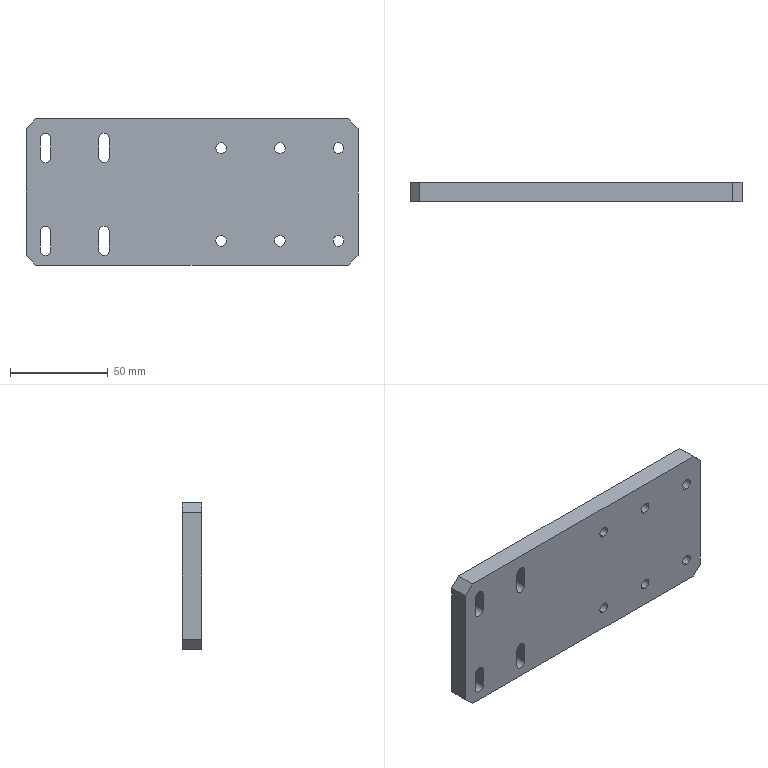Part | SolidWorks | features Chamfer 1, Cut 1, Extrusion 1 | 1 solid | 42 faces | box 170 x 10 x 75 mm | volume 122534 mm3 | cylinder 24 | plane 18 | commonest cylinder face diameters 5.5 x24
STEP:
#1=CARTESIAN_POINT('',(75.,0.,19.75));
#2=VERTEX_POINT('',#1);
#3=CARTESIAN_POINT('',(75.,0.,25.25));
#4=VERTEX_POINT('',#3);
#5=CARTESIAN_POINT('',(75.,0.,22.5));
#6=DIRECTION('',(0.,1.,0.));
#7=DIRECTION('',(0.,0.,1.));
#8=AXIS2_PLACEMENT_3D('',#5,#6,#7);
#9=CIRCLE('',#8,2.75);
#10=EDGE_CURVE('',#2,#4,#9,.T.);
#11=ORIENTED_EDGE('',*,*,#10,.F.);
#12=CARTESIAN_POINT('',(75.,10.,19.75));
#13=VERTEX_POINT('',#12);
#14=CARTESIAN_POINT('',(75.,-5.,19.75));
#15=DIRECTION('',(0.,1.,0.));
#16=VECTOR('',#15,1000.);
#17=LINE('',#14,#16);
#18=EDGE_CURVE('',#2,#13,#17,.T.);
#19=ORIENTED_EDGE('',*,*,#18,.T.);
#20=CARTESIAN_POINT('',(75.,10.,25.25));
#21=VERTEX_POINT('',#20);
#22=CARTESIAN_POINT('',(75.,10.,22.5));
#23=DIRECTION('',(0.,1.,0.));
#24=DIRECTION('',(0.,0.,1.));
#25=AXIS2_PLACEMENT_3D('',#22,#23,#24);
#26=CIRCLE('',#25,2.75);
#27=EDGE_CURVE('',#13,#21,#26,.T.);
#28=ORIENTED_EDGE('',*,*,#27,.T.);
#29=CARTESIAN_POINT('',(75.,-5.,25.25));
#30=DIRECTION('',(0.,1.,0.));
#31=VECTOR('',#30,1000.);
#32=LINE('',#29,#31);
#33=EDGE_CURVE('',#4,#21,#32,.T.);
#34=ORIENTED_EDGE('',*,*,#33,.F.);
#35=EDGE_LOOP('',(#11,#19,#28,#34));
#36=FACE_OUTER_BOUND('',#35,.T.);
#37=CARTESIAN_POINT('',(75.,-5.,22.5));
#38=DIRECTION('',(0.,1.,0.));
#39=DIRECTION('',(0.,0.,1.));
#40=AXIS2_PLACEMENT_3D('',#37,#38,#39);
#41=CYLINDRICAL_SURFACE('',#40,2.75);
#42=ADVANCED_FACE('',(#36),#41,.F.);
#43=CARTESIAN_POINT('',(-75.,0.,-17.5));
#44=VERTEX_POINT('',#43);
#45=CARTESIAN_POINT('',(-72.25,0.,-20.25));
#46=VERTEX_POINT('',#45);
#47=CARTESIAN_POINT('',(-75.,0.,-20.25));
#48=DIRECTION('',(0.,1.,0.));
#49=DIRECTION('',(0.,0.,1.));
#50=AXIS2_PLACEMENT_3D('',#47,#48,#49);
#51=CIRCLE('',#50,2.75);
#52=EDGE_CURVE('',#44,#46,#51,.T.);
#53=ORIENTED_EDGE('',*,*,#52,.F.);
#54=CARTESIAN_POINT('',(-75.,10.,-17.5));
#55=VERTEX_POINT('',#54);
#56=CARTESIAN_POINT('',(-75.,-5.,-17.5));
#57=DIRECTION('',(0.,1.,0.));
#58=VECTOR('',#57,1000.);
#59=LINE('',#56,#58);
#60=EDGE_CURVE('',#44,#55,#59,.T.);
#61=ORIENTED_EDGE('',*,*,#60,.T.);
#62=CARTESIAN_POINT('',(-72.25,10.,-20.25));
#63=VERTEX_POINT('',#62);
#64=CARTESIAN_POINT('',(-75.,10.,-20.25));
#65=DIRECTION('',(0.,1.,0.));
#66=DIRECTION('',(0.,0.,1.));
#67=AXIS2_PLACEMENT_3D('',#64,#65,#66);
#68=CIRCLE('',#67,2.75);
#69=EDGE_CURVE('',#55,#63,#68,.T.);
#70=ORIENTED_EDGE('',*,*,#69,.T.);
#71=CARTESIAN_POINT('',(-72.25,-5.,-20.25));
#72=DIRECTION('',(0.,1.,0.));
#73=VECTOR('',#72,1000.);
#74=LINE('',#71,#73);
#75=EDGE_CURVE('',#46,#63,#74,.T.);
#76=ORIENTED_EDGE('',*,*,#75,.F.);
#77=EDGE_LOOP('',(#53,#61,#70,#76));
#78=FACE_OUTER_BOUND('',#77,.T.);
#79=CARTESIAN_POINT('',(-75.,-5.,-20.25));
#80=DIRECTION('',(0.,1.,0.));
#81=DIRECTION('',(0.,0.,1.));
#82=AXIS2_PLACEMENT_3D('',#79,#80,#81);
#83=CYLINDRICAL_SURFACE('',#82,2.75);
#84=ADVANCED_FACE('',(#78),#83,.F.);
#85=CARTESIAN_POINT('',(-45.,0.,-17.5));
#86=VERTEX_POINT('',#85);
#87=CARTESIAN_POINT('',(-42.25,0.,-20.25));
#88=VERTEX_POINT('',#87);
#89=CARTESIAN_POINT('',(-45.,0.,-20.25));
#90=DIRECTION('',(0.,1.,0.));
#91=DIRECTION('',(0.,0.,1.));
#92=AXIS2_PLACEMENT_3D('',#89,#90,#91);
#93=CIRCLE('',#92,2.75);
#94=EDGE_CURVE('',#86,#88,#93,.T.);
#95=ORIENTED_EDGE('',*,*,#94,.F.);
#96=CARTESIAN_POINT('',(-45.,10.,-17.5));
#97=VERTEX_POINT('',#96);
#98=CARTESIAN_POINT('',(-45.,-5.,-17.5));
#99=DIRECTION('',(0.,1.,0.));
#100=VECTOR('',#99,1000.);
#101=LINE('',#98,#100);
#102=EDGE_CURVE('',#86,#97,#101,.T.);
#103=ORIENTED_EDGE('',*,*,#102,.T.);
#104=CARTESIAN_POINT('',(-42.25,10.,-20.25));
#105=VERTEX_POINT('',#104);
#106=CARTESIAN_POINT('',(-45.,10.,-20.25));
#107=DIRECTION('',(0.,1.,0.));
#108=DIRECTION('',(0.,0.,1.));
#109=AXIS2_PLACEMENT_3D('',#106,#107,#108);
#110=CIRCLE('',#109,2.75);
#111=EDGE_CURVE('',#97,#105,#110,.T.);
#112=ORIENTED_EDGE('',*,*,#111,.T.);
#113=CARTESIAN_POINT('',(-42.25,-5.,-20.25));
#114=DIRECTION('',(0.,1.,0.));
#115=VECTOR('',#114,1000.);
#116=LINE('',#113,#115);
#117=EDGE_CURVE('',#88,#105,#116,.T.);
#118=ORIENTED_EDGE('',*,*,#117,.F.);
#119=EDGE_LOOP('',(#95,#103,#112,#118));
#120=FACE_OUTER_BOUND('',#119,.T.);
#121=CARTESIAN_POINT('',(-45.,-5.,-20.25));
#122=DIRECTION('',(0.,1.,0.));
#123=DIRECTION('',(0.,0.,1.));
#124=AXIS2_PLACEMENT_3D('',#121,#122,#123);
#125=CYLINDRICAL_SURFACE('',#124,2.75);
#126=ADVANCED_FACE('',(#120),#125,.F.);
#127=CARTESIAN_POINT('',(-75.,0.,30.));
#128=VERTEX_POINT('',#127);
#129=CARTESIAN_POINT('',(-72.25,0.,27.25));
#130=VERTEX_POINT('',#129);
#131=CARTESIAN_POINT('',(-75.,0.,27.25));
#132=DIRECTION('',(0.,1.,0.));
#133=DIRECTION('',(0.,0.,1.));
#134=AXIS2_PLACEMENT_3D('',#131,#132,#133);
#135=CIRCLE('',#134,2.75);
#136=EDGE_CURVE('',#128,#130,#135,.T.);
#137=ORIENTED_EDGE('',*,*,#136,.F.);
#138=CARTESIAN_POINT('',(-75.,10.,30.));
#139=VERTEX_POINT('',#138);
#140=CARTESIAN_POINT('',(-75.,-5.,30.));
#141=DIRECTION('',(0.,1.,0.));
#142=VECTOR('',#141,1000.);
#143=LINE('',#140,#142);
#144=EDGE_CURVE('',#128,#139,#143,.T.);
#145=ORIENTED_EDGE('',*,*,#144,.T.);
#146=CARTESIAN_POINT('',(-72.25,10.,27.25));
#147=VERTEX_POINT('',#146);
#148=CARTESIAN_POINT('',(-75.,10.,27.25));
#149=DIRECTION('',(0.,1.,0.));
#150=DIRECTION('',(0.,0.,1.));
#151=AXIS2_PLACEMENT_3D('',#148,#149,#150);
#152=CIRCLE('',#151,2.75);
#153=EDGE_CURVE('',#139,#147,#152,.T.);
#154=ORIENTED_EDGE('',*,*,#153,.T.);
#155=CARTESIAN_POINT('',(-72.25,-5.,27.25));
#156=DIRECTION('',(0.,1.,0.));
#157=VECTOR('',#156,1000.);
#158=LINE('',#155,#157);
#159=EDGE_CURVE('',#130,#147,#158,.T.);
#160=ORIENTED_EDGE('',*,*,#159,.F.);
#161=EDGE_LOOP('',(#137,#145,#154,#160));
#162=FACE_OUTER_BOUND('',#161,.T.);
#163=CARTESIAN_POINT('',(-75.,-5.,27.25));
#164=DIRECTION('',(0.,1.,0.));
#165=DIRECTION('',(0.,0.,1.));
#166=AXIS2_PLACEMENT_3D('',#163,#164,#165);
#167=CYLINDRICAL_SURFACE('',#166,2.75);
#168=ADVANCED_FACE('',(#162),#167,.F.);
#169=CARTESIAN_POINT('',(45.,0.,19.75));
#170=VERTEX_POINT('',#169);
#171=CARTESIAN_POINT('',(45.,0.,25.25));
#172=VERTEX_POINT('',#171);
#173=CARTESIAN_POINT('',(45.,0.,22.5));
#174=DIRECTION('',(0.,1.,0.));
#175=DIRECTION('',(0.,0.,1.));
#176=AXIS2_PLACEMENT_3D('',#173,#174,#175);
#177=CIRCLE('',#176,2.75);
#178=EDGE_CURVE('',#170,#172,#177,.T.);
#179=ORIENTED_EDGE('',*,*,#178,.F.);
#180=CARTESIAN_POINT('',(45.,10.,19.75));
#181=VERTEX_POINT('',#180);
#182=CARTESIAN_POINT('',(45.,-5.,19.75));
#183=DIRECTION('',(0.,1.,0.));
#184=VECTOR('',#183,1000.);
#185=LINE('',#182,#184);
#186=EDGE_CURVE('',#170,#181,#185,.T.);
#187=ORIENTED_EDGE('',*,*,#186,.T.);
#188=CARTESIAN_POINT('',(45.,10.,25.25));
#189=VERTEX_POINT('',#188);
#190=CARTESIAN_POINT('',(45.,10.,22.5));
#191=DIRECTION('',(0.,1.,0.));
#192=DIRECTION('',(0.,0.,1.));
#193=AXIS2_PLACEMENT_3D('',#190,#191,#192);
#194=CIRCLE('',#193,2.75);
#195=EDGE_CURVE('',#181,#189,#194,.T.);
#196=ORIENTED_EDGE('',*,*,#195,.T.);
#197=CARTESIAN_POINT('',(45.,-5.,25.25));
#198=DIRECTION('',(0.,1.,0.));
#199=VECTOR('',#198,1000.);
#200=LINE('',#197,#199);
#201=EDGE_CURVE('',#172,#189,#200,.T.);
#202=ORIENTED_EDGE('',*,*,#201,.F.);
#203=EDGE_LOOP('',(#179,#187,#196,#202));
#204=FACE_OUTER_BOUND('',#203,.T.);
#205=CARTESIAN_POINT('',(45.,-5.,22.5));
#206=DIRECTION('',(0.,1.,0.));
#207=DIRECTION('',(0.,0.,1.));
#208=AXIS2_PLACEMENT_3D('',#205,#206,#207);
#209=CYLINDRICAL_SURFACE('',#208,2.75);
#210=ADVANCED_FACE('',(#204),#209,.F.);
#211=CARTESIAN_POINT('',(15.,0.,19.75));
#212=VERTEX_POINT('',#211);
#213=CARTESIAN_POINT('',(15.,0.,25.25));
#214=VERTEX_POINT('',#213);
#215=CARTESIAN_POINT('',(15.,0.,22.5));
#216=DIRECTION('',(0.,1.,0.));
#217=DIRECTION('',(0.,0.,1.));
#218=AXIS2_PLACEMENT_3D('',#215,#216,#217);
#219=CIRCLE('',#218,2.75);
#220=EDGE_CURVE('',#212,#214,#219,.T.);
#221=ORIENTED_EDGE('',*,*,#220,.F.);
#222=CARTESIAN_POINT('',(15.,10.,19.75));
#223=VERTEX_POINT('',#222);
#224=CARTESIAN_POINT('',(15.,-5.,19.75));
#225=DIRECTION('',(0.,1.,0.));
#226=VECTOR('',#225,1000.);
#227=LINE('',#224,#226);
#228=EDGE_CURVE('',#212,#223,#227,.T.);
#229=ORIENTED_EDGE('',*,*,#228,.T.);
#230=CARTESIAN_POINT('',(15.,10.,25.25));
#231=VERTEX_POINT('',#230);
#232=CARTESIAN_POINT('',(15.,10.,22.5));
#233=DIRECTION('',(0.,1.,0.));
#234=DIRECTION('',(0.,0.,1.));
#235=AXIS2_PLACEMENT_3D('',#232,#233,#234);
#236=CIRCLE('',#235,2.75);
#237=EDGE_CURVE('',#223,#231,#236,.T.);
#238=ORIENTED_EDGE('',*,*,#237,.T.);
#239=CARTESIAN_POINT('',(15.,-5.,25.25));
#240=DIRECTION('',(0.,1.,0.));
#241=VECTOR('',#240,1000.);
#242=LINE('',#239,#241);
#243=EDGE_CURVE('',#214,#231,#242,.T.);
#244=ORIENTED_EDGE('',*,*,#243,.F.);
#245=EDGE_LOOP('',(#221,#229,#238,#244));
#246=FACE_OUTER_BOUND('',#245,.T.);
#247=CARTESIAN_POINT('',(15.,-5.,22.5));
#248=DIRECTION('',(0.,1.,0.));
#249=DIRECTION('',(0.,0.,1.));
#250=AXIS2_PLACEMENT_3D('',#247,#248,#249);
#251=CYLINDRICAL_SURFACE('',#250,2.75);
#252=ADVANCED_FACE('',(#246),#251,.F.);
#253=CARTESIAN_POINT('',(75.,0.,-27.75));
#254=VERTEX_POINT('',#253);
#255=CARTESIAN_POINT('',(75.,0.,-22.25));
#256=VERTEX_POINT('',#255);
#257=CARTESIAN_POINT('',(75.,0.,-25.));
#258=DIRECTION('',(0.,1.,0.));
#259=DIRECTION('',(0.,0.,1.));
#260=AXIS2_PLACEMENT_3D('',#257,#258,#259);
#261=CIRCLE('',#260,2.75);
#262=EDGE_CURVE('',#254,#256,#261,.T.);
#263=ORIENTED_EDGE('',*,*,#262,.F.);
#264=CARTESIAN_POINT('',(75.,10.,-27.75));
#265=VERTEX_POINT('',#264);
#266=CARTESIAN_POINT('',(75.,-5.,-27.75));
#267=DIRECTION('',(0.,1.,0.));
#268=VECTOR('',#267,1000.);
#269=LINE('',#266,#268);
#270=EDGE_CURVE('',#254,#265,#269,.T.);
#271=ORIENTED_EDGE('',*,*,#270,.T.);
#272=CARTESIAN_POINT('',(75.,10.,-22.25));
#273=VERTEX_POINT('',#272);
#274=CARTESIAN_POINT('',(75.,10.,-25.));
#275=DIRECTION('',(0.,1.,0.));
#276=DIRECTION('',(0.,0.,1.));
#277=AXIS2_PLACEMENT_3D('',#274,#275,#276);
#278=CIRCLE('',#277,2.75);
#279=EDGE_CURVE('',#265,#273,#278,.T.);
#280=ORIENTED_EDGE('',*,*,#279,.T.);
#281=CARTESIAN_POINT('',(75.,-5.,-22.25));
#282=DIRECTION('',(0.,1.,0.));
#283=VECTOR('',#282,1000.);
#284=LINE('',#281,#283);
#285=EDGE_CURVE('',#256,#273,#284,.T.);
#286=ORIENTED_EDGE('',*,*,#285,.F.);
#287=EDGE_LOOP('',(#263,#271,#280,#286));
#288=FACE_OUTER_BOUND('',#287,.T.);
#289=CARTESIAN_POINT('',(75.,-5.,-25.));
#290=DIRECTION('',(0.,1.,0.));
#291=DIRECTION('',(0.,0.,1.));
#292=AXIS2_PLACEMENT_3D('',#289,#290,#291);
#293=CYLINDRICAL_SURFACE('',#292,2.75);
#294=ADVANCED_FACE('',(#288),#293,.F.);
#295=CARTESIAN_POINT('',(45.,0.,-27.75));
#296=VERTEX_POINT('',#295);
#297=CARTESIAN_POINT('',(45.,0.,-22.25));
#298=VERTEX_POINT('',#297);
#299=CARTESIAN_POINT('',(45.,0.,-25.));
#300=DIRECTION('',(0.,1.,0.));
#301=DIRECTION('',(0.,0.,1.));
#302=AXIS2_PLACEMENT_3D('',#299,#300,#301);
#303=CIRCLE('',#302,2.75);
#304=EDGE_CURVE('',#296,#298,#303,.T.);
#305=ORIENTED_EDGE('',*,*,#304,.F.);
#306=CARTESIAN_POINT('',(45.,10.,-27.75));
#307=VERTEX_POINT('',#306);
#308=CARTESIAN_POINT('',(45.,-5.,-27.75));
#309=DIRECTION('',(0.,1.,0.));
#310=VECTOR('',#309,1000.);
#311=LINE('',#308,#310);
#312=EDGE_CURVE('',#296,#307,#311,.T.);
#313=ORIENTED_EDGE('',*,*,#312,.T.);
#314=CARTESIAN_POINT('',(45.,10.,-22.25));
#315=VERTEX_POINT('',#314);
#316=CARTESIAN_POINT('',(45.,10.,-25.));
#317=DIRECTION('',(0.,1.,0.));
#318=DIRECTION('',(0.,0.,1.));
#319=AXIS2_PLACEMENT_3D('',#316,#317,#318);
#320=CIRCLE('',#319,2.75);
#321=EDGE_CURVE('',#307,#315,#320,.T.);
#322=ORIENTED_EDGE('',*,*,#321,.T.);
#323=CARTESIAN_POINT('',(45.,-5.,-22.25));
#324=DIRECTION('',(0.,1.,0.));
#325=VECTOR('',#324,1000.);
#326=LINE('',#323,#325);
#327=EDGE_CURVE('',#298,#315,#326,.T.);
#328=ORIENTED_EDGE('',*,*,#327,.F.);
#329=EDGE_LOOP('',(#305,#313,#322,#328));
#330=FACE_OUTER_BOUND('',#329,.T.);
#331=CARTESIAN_POINT('',(45.,-5.,-25.));
#332=DIRECTION('',(0.,1.,0.));
#333=DIRECTION('',(0.,0.,1.));
#334=AXIS2_PLACEMENT_3D('',#331,#332,#333);
#335=CYLINDRICAL_SURFACE('',#334,2.75);
#336=ADVANCED_FACE('',(#330),#335,.F.);
#337=CARTESIAN_POINT('',(-45.,0.,30.));
#338=VERTEX_POINT('',#337);
#339=CARTESIAN_POINT('',(-42.25,0.,27.25));
#340=VERTEX_POINT('',#339);
#341=CARTESIAN_POINT('',(-45.,0.,27.25));
#342=DIRECTION('',(0.,1.,0.));
#343=DIRECTION('',(0.,0.,1.));
#344=AXIS2_PLACEMENT_3D('',#341,#342,#343);
#345=CIRCLE('',#344,2.75);
#346=EDGE_CURVE('',#338,#340,#345,.T.);
#347=ORIENTED_EDGE('',*,*,#346,.F.);
#348=CARTESIAN_POINT('',(-45.,10.,30.));
#349=VERTEX_POINT('',#348);
#350=CARTESIAN_POINT('',(-45.,-5.,30.));
#351=DIRECTION('',(0.,1.,0.));
#352=VECTOR('',#351,1000.);
#353=LINE('',#350,#352);
#354=EDGE_CURVE('',#338,#349,#353,.T.);
#355=ORIENTED_EDGE('',*,*,#354,.T.);
#356=CARTESIAN_POINT('',(-42.25,10.,27.25));
#357=VERTEX_POINT('',#356);
#358=CARTESIAN_POINT('',(-45.,10.,27.25));
#359=DIRECTION('',(0.,1.,0.));
#360=DIRECTION('',(0.,0.,1.));
#361=AXIS2_PLACEMENT_3D('',#358,#359,#360);
#362=CIRCLE('',#361,2.75);
#363=EDGE_CURVE('',#349,#357,#362,.T.);
#364=ORIENTED_EDGE('',*,*,#363,.T.);
#365=CARTESIAN_POINT('',(-42.25,-5.,27.25));
#366=DIRECTION('',(0.,1.,0.));
#367=VECTOR('',#366,1000.);
#368=LINE('',#365,#367);
#369=EDGE_CURVE('',#340,#357,#368,.T.);
#370=ORIENTED_EDGE('',*,*,#369,.F.);
#371=EDGE_LOOP('',(#347,#355,#364,#370));
#372=FACE_OUTER_BOUND('',#371,.T.);
#373=CARTESIAN_POINT('',(-45.,-5.,27.25));
#374=DIRECTION('',(0.,1.,0.));
#375=DIRECTION('',(0.,0.,1.));
#376=AXIS2_PLACEMENT_3D('',#373,#374,#375);
#377=CYLINDRICAL_SURFACE('',#376,2.75);
#378=ADVANCED_FACE('',(#372),#377,.F.);
#379=CARTESIAN_POINT('',(15.,0.,-27.75));
#380=VERTEX_POINT('',#379);
#381=CARTESIAN_POINT('',(15.,0.,-22.25));
#382=VERTEX_POINT('',#381);
#383=CARTESIAN_POINT('',(15.,0.,-25.));
#384=DIRECTION('',(0.,1.,0.));
#385=DIRECTION('',(0.,0.,1.));
#386=AXIS2_PLACEMENT_3D('',#383,#384,#385);
#387=CIRCLE('',#386,2.75);
#388=EDGE_CURVE('',#380,#382,#387,.T.);
#389=ORIENTED_EDGE('',*,*,#388,.F.);
#390=CARTESIAN_POINT('',(15.,10.,-27.75));
#391=VERTEX_POINT('',#390);
#392=CARTESIAN_POINT('',(15.,-5.,-27.75));
#393=DIRECTION('',(0.,1.,0.));
#394=VECTOR('',#393,1000.);
#395=LINE('',#392,#394);
#396=EDGE_CURVE('',#380,#391,#395,.T.);
#397=ORIENTED_EDGE('',*,*,#396,.T.);
#398=CARTESIAN_POINT('',(15.,10.,-22.25));
#399=VERTEX_POINT('',#398);
#400=CARTESIAN_POINT('',(15.,10.,-25.));
#401=DIRECTION('',(0.,1.,0.));
#402=DIRECTION('',(0.,0.,1.));
#403=AXIS2_PLACEMENT_3D('',#400,#401,#402);
#404=CIRCLE('',#403,2.75);
#405=EDGE_CURVE('',#391,#399,#404,.T.);
#406=ORIENTED_EDGE('',*,*,#405,.T.);
#407=CARTESIAN_POINT('',(15.,-5.,-22.25));
#408=DIRECTION('',(0.,1.,0.));
#409=VECTOR('',#408,1000.);
#410=LINE('',#407,#409);
#411=EDGE_CURVE('',#382,#399,#410,.T.);
#412=ORIENTED_EDGE('',*,*,#411,.F.);
#413=EDGE_LOOP('',(#389,#397,#406,#412));
#414=FACE_OUTER_BOUND('',#413,.T.);
#415=CARTESIAN_POINT('',(15.,-5.,-25.));
#416=DIRECTION('',(0.,1.,0.));
#417=DIRECTION('',(0.,0.,1.));
#418=AXIS2_PLACEMENT_3D('',#415,#416,#417);
#419=CYLINDRICAL_SURFACE('',#418,2.75);
#420=ADVANCED_FACE('',(#414),#419,.F.);
#421=CARTESIAN_POINT('',(85.,0.,32.5));
#422=VERTEX_POINT('',#421);
#423=CARTESIAN_POINT('',(85.,0.,-32.5));
#424=VERTEX_POINT('',#423);
#425=CARTESIAN_POINT('',(85.,0.,-37.5));
#426=DIRECTION('',(0.,0.,-1.));
#427=VECTOR('',#426,1000.);
#428=LINE('',#425,#427);
#429=EDGE_CURVE('',#422,#424,#428,.T.);
#430=ORIENTED_EDGE('',*,*,#429,.T.);
#431=CARTESIAN_POINT('',(85.,10.,-32.5));
#432=VERTEX_POINT('',#431);
#433=CARTESIAN_POINT('',(85.,10.,-32.5));
#434=DIRECTION('',(0.,1.,0.));
#435=VECTOR('',#434,1000.);
#436=LINE('',#433,#435);
#437=EDGE_CURVE('',#424,#432,#436,.T.);
#438=ORIENTED_EDGE('',*,*,#437,.T.);
#439=CARTESIAN_POINT('',(85.,10.,32.5));
#440=VERTEX_POINT('',#439);
#441=CARTESIAN_POINT('',(85.,10.,-37.5));
#442=DIRECTION('',(0.,0.,-1.));
#443=VECTOR('',#442,1000.);
#444=LINE('',#441,#443);
#445=EDGE_CURVE('',#440,#432,#444,.T.);
#446=ORIENTED_EDGE('',*,*,#445,.F.);
#447=CARTESIAN_POINT('',(85.,10.,32.5));
#448=DIRECTION('',(0.,-1.,0.));
#449=VECTOR('',#448,1000.);
#450=LINE('',#447,#449);
#451=EDGE_CURVE('',#440,#422,#450,.T.);
#452=ORIENTED_EDGE('',*,*,#451,.T.);
#453=EDGE_LOOP('',(#430,#438,#446,#452));
#454=FACE_OUTER_BOUND('',#453,.T.);
#455=CARTESIAN_POINT('',(85.,10.,-37.5));
#456=DIRECTION('',(-1.,0.,0.));
#457=DIRECTION('',(0.,0.,1.));
#458=AXIS2_PLACEMENT_3D('',#455,#456,#457);
#459=PLANE('',#458);
#460=ADVANCED_FACE('',(#454),#459,.F.);
#461=CARTESIAN_POINT('',(80.,0.,-37.5));
#462=VERTEX_POINT('',#461);
#463=CARTESIAN_POINT('',(-80.,0.,-37.5));
#464=VERTEX_POINT('',#463);
#465=CARTESIAN_POINT('',(-85.,0.,-37.5));
#466=DIRECTION('',(-1.,0.,0.));
#467=VECTOR('',#466,1000.);
#468=LINE('',#465,#467);
#469=EDGE_CURVE('',#462,#464,#468,.T.);
#470=ORIENTED_EDGE('',*,*,#469,.T.);
#471=CARTESIAN_POINT('',(-80.,10.,-37.5));
#472=VERTEX_POINT('',#471);
#473=CARTESIAN_POINT('',(-80.,10.,-37.5));
#474=DIRECTION('',(0.,1.,0.));
#475=VECTOR('',#474,1000.);
#476=LINE('',#473,#475);
#477=EDGE_CURVE('',#464,#472,#476,.T.);
#478=ORIENTED_EDGE('',*,*,#477,.T.);
#479=CARTESIAN_POINT('',(80.,10.,-37.5));
#480=VERTEX_POINT('',#479);
#481=CARTESIAN_POINT('',(-85.,10.,-37.5));
#482=DIRECTION('',(-1.,0.,0.));
#483=VECTOR('',#482,1000.);
#484=LINE('',#481,#483);
#485=EDGE_CURVE('',#480,#472,#484,.T.);
#486=ORIENTED_EDGE('',*,*,#485,.F.);
#487=CARTESIAN_POINT('',(80.,10.,-37.5));
#488=DIRECTION('',(0.,-1.,0.));
#489=VECTOR('',#488,1000.);
#490=LINE('',#487,#489);
#491=EDGE_CURVE('',#480,#462,#490,.T.);
#492=ORIENTED_EDGE('',*,*,#491,.T.);
#493=EDGE_LOOP('',(#470,#478,#486,#492));
#494=FACE_OUTER_BOUND('',#493,.T.);
#495=CARTESIAN_POINT('',(-85.,10.,-37.5));
#496=DIRECTION('',(0.,0.,1.));
#497=DIRECTION('',(1.,0.,0.));
#498=AXIS2_PLACEMENT_3D('',#495,#496,#497);
#499=PLANE('',#498);
#500=ADVANCED_FACE('',(#494),#499,.F.);
#501=CARTESIAN_POINT('',(-85.,10.,-32.5));
#502=VERTEX_POINT('',#501);
#503=CARTESIAN_POINT('',(-85.,10.,32.5));
#504=VERTEX_POINT('',#503);
#505=CARTESIAN_POINT('',(-85.,10.,-37.5));
#506=DIRECTION('',(0.,0.,1.));
#507=VECTOR('',#506,1000.);
#508=LINE('',#505,#507);
#509=EDGE_CURVE('',#502,#504,#508,.T.);
#510=ORIENTED_EDGE('',*,*,#509,.F.);
#511=CARTESIAN_POINT('',(-85.,0.,-32.5));
#512=VERTEX_POINT('',#511);
#513=CARTESIAN_POINT('',(-85.,10.,-32.5));
#514=DIRECTION('',(0.,-1.,0.));
#515=VECTOR('',#514,1000.);
#516=LINE('',#513,#515);
#517=EDGE_CURVE('',#502,#512,#516,.T.);
#518=ORIENTED_EDGE('',*,*,#517,.T.);
#519=CARTESIAN_POINT('',(-85.,0.,32.5));
#520=VERTEX_POINT('',#519);
#521=CARTESIAN_POINT('',(-85.,0.,-37.5));
#522=DIRECTION('',(0.,0.,1.));
#523=VECTOR('',#522,1000.);
#524=LINE('',#521,#523);
#525=EDGE_CURVE('',#512,#520,#524,.T.);
#526=ORIENTED_EDGE('',*,*,#525,.T.);
#527=CARTESIAN_POINT('',(-85.,10.,32.5));
#528=DIRECTION('',(0.,1.,0.));
#529=VECTOR('',#528,1000.);
#530=LINE('',#527,#529);
#531=EDGE_CURVE('',#520,#504,#530,.T.);
#532=ORIENTED_EDGE('',*,*,#531,.T.);
#533=EDGE_LOOP('',(#510,#518,#526,#532));
#534=FACE_OUTER_BOUND('',#533,.T.);
#535=CARTESIAN_POINT('',(-85.,10.,-37.5));
#536=DIRECTION('',(1.,0.,0.));
#537=DIRECTION('',(0.,0.,-1.));
#538=AXIS2_PLACEMENT_3D('',#535,#536,#537);
#539=PLANE('',#538);
#540=ADVANCED_FACE('',(#534),#539,.F.);
#541=CARTESIAN_POINT('',(-80.,0.,37.5));
#542=VERTEX_POINT('',#541);
#543=CARTESIAN_POINT('',(80.,0.,37.5));
#544=VERTEX_POINT('',#543);
#545=CARTESIAN_POINT('',(-85.,0.,37.5));
#546=DIRECTION('',(1.,0.,0.));
#547=VECTOR('',#546,1000.);
#548=LINE('',#545,#547);
#549=EDGE_CURVE('',#542,#544,#548,.T.);
#550=ORIENTED_EDGE('',*,*,#549,.T.);
#551=CARTESIAN_POINT('',(80.,10.,37.5));
#552=VERTEX_POINT('',#551);
#553=CARTESIAN_POINT('',(80.,10.,37.5));
#554=DIRECTION('',(0.,1.,0.));
#555=VECTOR('',#554,1000.);
#556=LINE('',#553,#555);
#557=EDGE_CURVE('',#544,#552,#556,.T.);
#558=ORIENTED_EDGE('',*,*,#557,.T.);
#559=CARTESIAN_POINT('',(-80.,10.,37.5));
#560=VERTEX_POINT('',#559);
#561=CARTESIAN_POINT('',(-85.,10.,37.5));
#562=DIRECTION('',(1.,0.,0.));
#563=VECTOR('',#562,1000.);
#564=LINE('',#561,#563);
#565=EDGE_CURVE('',#560,#552,#564,.T.);
#566=ORIENTED_EDGE('',*,*,#565,.F.);
#567=CARTESIAN_POINT('',(-80.,10.,37.5));
#568=DIRECTION('',(0.,-1.,0.));
#569=VECTOR('',#568,1000.);
#570=LINE('',#567,#569);
#571=EDGE_CURVE('',#560,#542,#570,.T.);
#572=ORIENTED_EDGE('',*,*,#571,.T.);
#573=EDGE_LOOP('',(#550,#558,#566,#572));
#574=FACE_OUTER_BOUND('',#573,.T.);
#575=CARTESIAN_POINT('',(-85.,10.,37.5));
#576=DIRECTION('',(0.,0.,-1.));
#577=DIRECTION('',(-1.,0.,0.));
#578=AXIS2_PLACEMENT_3D('',#575,#576,#577);
#579=PLANE('',#578);
#580=ADVANCED_FACE('',(#574),#579,.F.);
#581=CARTESIAN_POINT('',(75.,10.,22.5));
#582=DIRECTION('',(0.,1.,0.));
#583=DIRECTION('',(0.,0.,1.));
#584=AXIS2_PLACEMENT_3D('',#581,#582,#583);
#585=CIRCLE('',#584,2.75);
#586=EDGE_CURVE('',#21,#13,#585,.T.);
#587=ORIENTED_EDGE('',*,*,#586,.F.);
#588=ORIENTED_EDGE('',*,*,#27,.F.);
#589=EDGE_LOOP('',(#587,#588));
#590=FACE_BOUND('',#589,.T.);
#591=CARTESIAN_POINT('',(-72.25,10.,-29.75));
#592=VERTEX_POINT('',#591);
#593=CARTESIAN_POINT('',(-77.75,10.,-29.75));
#594=VERTEX_POINT('',#593);
#595=CARTESIAN_POINT('',(-75.,10.,-29.75));
#596=DIRECTION('',(0.,1.,0.));
#597=DIRECTION('',(0.,0.,1.));
#598=AXIS2_PLACEMENT_3D('',#595,#596,#597);
#599=CIRCLE('',#598,2.75);
#600=EDGE_CURVE('',#592,#594,#599,.T.);
#601=ORIENTED_EDGE('',*,*,#600,.F.);
#602=CARTESIAN_POINT('',(-72.25,10.,-29.75));
#603=DIRECTION('',(0.,0.,-1.));
#604=VECTOR('',#603,1000.);
#605=LINE('',#602,#604);
#606=EDGE_CURVE('',#63,#592,#605,.T.);
#607=ORIENTED_EDGE('',*,*,#606,.F.);
#608=ORIENTED_EDGE('',*,*,#69,.F.);
#609=CARTESIAN_POINT('',(-77.75,10.,-20.25));
#610=VERTEX_POINT('',#609);
#611=CARTESIAN_POINT('',(-75.,10.,-20.25));
#612=DIRECTION('',(0.,1.,0.));
#613=DIRECTION('',(0.,0.,1.));
#614=AXIS2_PLACEMENT_3D('',#611,#612,#613);
#615=CIRCLE('',#614,2.75);
#616=EDGE_CURVE('',#610,#55,#615,.T.);
#617=ORIENTED_EDGE('',*,*,#616,.F.);
#618=CARTESIAN_POINT('',(-77.75,10.,-29.75));
#619=DIRECTION('',(0.,0.,1.));
#620=VECTOR('',#619,1000.);
#621=LINE('',#618,#620);
#622=EDGE_CURVE('',#594,#610,#621,.T.);
#623=ORIENTED_EDGE('',*,*,#622,.F.);
#624=EDGE_LOOP('',(#601,#607,#608,#617,#623));
#625=FACE_BOUND('',#624,.T.);
#626=CARTESIAN_POINT('',(-42.25,10.,-29.75));
#627=VERTEX_POINT('',#626);
#628=CARTESIAN_POINT('',(-47.75,10.,-29.75));
#629=VERTEX_POINT('',#628);
#630=CARTESIAN_POINT('',(-45.,10.,-29.75));
#631=DIRECTION('',(0.,1.,0.));
#632=DIRECTION('',(0.,0.,1.));
#633=AXIS2_PLACEMENT_3D('',#630,#631,#632);
#634=CIRCLE('',#633,2.75);
#635=EDGE_CURVE('',#627,#629,#634,.T.);
#636=ORIENTED_EDGE('',*,*,#635,.F.);
#637=CARTESIAN_POINT('',(-42.25,10.,-29.75));
#638=DIRECTION('',(0.,0.,-1.));
#639=VECTOR('',#638,1000.);
#640=LINE('',#637,#639);
#641=EDGE_CURVE('',#105,#627,#640,.T.);
#642=ORIENTED_EDGE('',*,*,#641,.F.);
#643=ORIENTED_EDGE('',*,*,#111,.F.);
#644=CARTESIAN_POINT('',(-47.75,10.,-20.25));
#645=VERTEX_POINT('',#644);
#646=CARTESIAN_POINT('',(-45.,10.,-20.25));
#647=DIRECTION('',(0.,1.,0.));
#648=DIRECTION('',(0.,0.,1.));
#649=AXIS2_PLACEMENT_3D('',#646,#647,#648);
#650=CIRCLE('',#649,2.75);
#651=EDGE_CURVE('',#645,#97,#650,.T.);
#652=ORIENTED_EDGE('',*,*,#651,.F.);
#653=CARTESIAN_POINT('',(-47.75,10.,-29.75));
#654=DIRECTION('',(0.,0.,1.));
#655=VECTOR('',#654,1000.);
#656=LINE('',#653,#655);
#657=EDGE_CURVE('',#629,#645,#656,.T.);
#658=ORIENTED_EDGE('',*,*,#657,.F.);
#659=EDGE_LOOP('',(#636,#642,#643,#652,#658));
#660=FACE_BOUND('',#659,.T.);
#661=CARTESIAN_POINT('',(-72.25,10.,17.75));
#662=VERTEX_POINT('',#661);
#663=CARTESIAN_POINT('',(-77.75,10.,17.75));
#664=VERTEX_POINT('',#663);
#665=CARTESIAN_POINT('',(-75.,10.,17.75));
#666=DIRECTION('',(0.,1.,0.));
#667=DIRECTION('',(0.,0.,1.));
#668=AXIS2_PLACEMENT_3D('',#665,#666,#667);
#669=CIRCLE('',#668,2.75);
#670=EDGE_CURVE('',#662,#664,#669,.T.);
#671=ORIENTED_EDGE('',*,*,#670,.F.);
#672=CARTESIAN_POINT('',(-72.25,10.,17.75));
#673=DIRECTION('',(0.,0.,-1.));
#674=VECTOR('',#673,1000.);
#675=LINE('',#672,#674);
#676=EDGE_CURVE('',#147,#662,#675,.T.);
#677=ORIENTED_EDGE('',*,*,#676,.F.);
#678=ORIENTED_EDGE('',*,*,#153,.F.);
#679=CARTESIAN_POINT('',(-77.75,10.,27.25));
#680=VERTEX_POINT('',#679);
#681=CARTESIAN_POINT('',(-75.,10.,27.25));
#682=DIRECTION('',(0.,1.,0.));
#683=DIRECTION('',(0.,0.,1.));
#684=AXIS2_PLACEMENT_3D('',#681,#682,#683);
#685=CIRCLE('',#684,2.75);
#686=EDGE_CURVE('',#680,#139,#685,.T.);
#687=ORIENTED_EDGE('',*,*,#686,.F.);
#688=CARTESIAN_POINT('',(-77.75,10.,17.75));
#689=DIRECTION('',(0.,0.,1.));
#690=VECTOR('',#689,1000.);
#691=LINE('',#688,#690);
#692=EDGE_CURVE('',#664,#680,#691,.T.);
#693=ORIENTED_EDGE('',*,*,#692,.F.);
#694=EDGE_LOOP('',(#671,#677,#678,#687,#693));
#695=FACE_BOUND('',#694,.T.);
#696=CARTESIAN_POINT('',(45.,10.,22.5));
#697=DIRECTION('',(0.,1.,0.));
#698=DIRECTION('',(0.,0.,1.));
#699=AXIS2_PLACEMENT_3D('',#696,#697,#698);
#700=CIRCLE('',#699,2.75);
#701=EDGE_CURVE('',#189,#181,#700,.T.);
#702=ORIENTED_EDGE('',*,*,#701,.F.);
#703=ORIENTED_EDGE('',*,*,#195,.F.);
#704=EDGE_LOOP('',(#702,#703));
#705=FACE_BOUND('',#704,.T.);
#706=CARTESIAN_POINT('',(15.,10.,22.5));
#707=DIRECTION('',(0.,1.,0.));
#708=DIRECTION('',(0.,0.,1.));
#709=AXIS2_PLACEMENT_3D('',#706,#707,#708);
#710=CIRCLE('',#709,2.75);
#711=EDGE_CURVE('',#231,#223,#710,.T.);
#712=ORIENTED_EDGE('',*,*,#711,.F.);
#713=ORIENTED_EDGE('',*,*,#237,.F.);
#714=EDGE_LOOP('',(#712,#713));
#715=FACE_BOUND('',#714,.T.);
#716=CARTESIAN_POINT('',(75.,10.,-25.));
#717=DIRECTION('',(0.,1.,0.));
#718=DIRECTION('',(0.,0.,1.));
#719=AXIS2_PLACEMENT_3D('',#716,#717,#718);
#720=CIRCLE('',#719,2.75);
#721=EDGE_CURVE('',#273,#265,#720,.T.);
#722=ORIENTED_EDGE('',*,*,#721,.F.);
#723=ORIENTED_EDGE('',*,*,#279,.F.);
#724=EDGE_LOOP('',(#722,#723));
#725=FACE_BOUND('',#724,.T.);
#726=CARTESIAN_POINT('',(45.,10.,-25.));
#727=DIRECTION('',(0.,1.,0.));
#728=DIRECTION('',(0.,0.,1.));
#729=AXIS2_PLACEMENT_3D('',#726,#727,#728);
#730=CIRCLE('',#729,2.75);
#731=EDGE_CURVE('',#315,#307,#730,.T.);
#732=ORIENTED_EDGE('',*,*,#731,.F.);
#733=ORIENTED_EDGE('',*,*,#321,.F.);
#734=EDGE_LOOP('',(#732,#733));
#735=FACE_BOUND('',#734,.T.);
#736=CARTESIAN_POINT('',(-42.25,10.,17.75));
#737=VERTEX_POINT('',#736);
#738=CARTESIAN_POINT('',(-47.75,10.,17.75));
#739=VERTEX_POINT('',#738);
#740=CARTESIAN_POINT('',(-45.,10.,17.75));
#741=DIRECTION('',(0.,1.,0.));
#742=DIRECTION('',(0.,0.,1.));
#743=AXIS2_PLACEMENT_3D('',#740,#741,#742);
#744=CIRCLE('',#743,2.75);
#745=EDGE_CURVE('',#737,#739,#744,.T.);
#746=ORIENTED_EDGE('',*,*,#745,.F.);
#747=CARTESIAN_POINT('',(-42.25,10.,17.75));
#748=DIRECTION('',(0.,0.,-1.));
#749=VECTOR('',#748,1000.);
#750=LINE('',#747,#749);
#751=EDGE_CURVE('',#357,#737,#750,.T.);
#752=ORIENTED_EDGE('',*,*,#751,.F.);
#753=ORIENTED_EDGE('',*,*,#363,.F.);
#754=CARTESIAN_POINT('',(-47.75,10.,27.25));
#755=VERTEX_POINT('',#754);
#756=CARTESIAN_POINT('',(-45.,10.,27.25));
#757=DIRECTION('',(0.,1.,0.));
#758=DIRECTION('',(0.,0.,1.));
#759=AXIS2_PLACEMENT_3D('',#756,#757,#758);
#760=CIRCLE('',#759,2.75);
#761=EDGE_CURVE('',#755,#349,#760,.T.);
#762=ORIENTED_EDGE('',*,*,#761,.F.);
#763=CARTESIAN_POINT('',(-47.75,10.,17.75));
#764=DIRECTION('',(0.,0.,1.));
#765=VECTOR('',#764,1000.);
#766=LINE('',#763,#765);
#767=EDGE_CURVE('',#739,#755,#766,.T.);
#768=ORIENTED_EDGE('',*,*,#767,.F.);
#769=EDGE_LOOP('',(#746,#752,#753,#762,#768));
#770=FACE_BOUND('',#769,.T.);
#771=CARTESIAN_POINT('',(15.,10.,-25.));
#772=DIRECTION('',(0.,1.,0.));
#773=DIRECTION('',(0.,0.,1.));
#774=AXIS2_PLACEMENT_3D('',#771,#772,#773);
#775=CIRCLE('',#774,2.75);
#776=EDGE_CURVE('',#399,#391,#775,.T.);
#777=ORIENTED_EDGE('',*,*,#776,.F.);
#778=ORIENTED_EDGE('',*,*,#405,.F.);
#779=EDGE_LOOP('',(#777,#778));
#780=FACE_BOUND('',#779,.T.);
#781=ORIENTED_EDGE('',*,*,#485,.T.);
#782=CARTESIAN_POINT('',(-58.75,10.,-58.75));
#783=DIRECTION('',(-0.7071,0.,0.7071));
#784=VECTOR('',#783,1000.);
#785=LINE('',#782,#784);
#786=EDGE_CURVE('',#472,#502,#785,.T.);
#787=ORIENTED_EDGE('',*,*,#786,.T.);
#788=ORIENTED_EDGE('',*,*,#509,.T.);
#789=CARTESIAN_POINT('',(-58.75,10.,58.75));
#790=DIRECTION('',(0.7071,0.,0.7071));
#791=VECTOR('',#790,1000.);
#792=LINE('',#789,#791);
#793=EDGE_CURVE('',#504,#560,#792,.T.);
#794=ORIENTED_EDGE('',*,*,#793,.T.);
#795=ORIENTED_EDGE('',*,*,#565,.T.);
#796=CARTESIAN_POINT('',(58.75,10.,58.75));
#797=DIRECTION('',(0.7071,0.,-0.7071));
#798=VECTOR('',#797,1000.);
#799=LINE('',#796,#798);
#800=EDGE_CURVE('',#552,#440,#799,.T.);
#801=ORIENTED_EDGE('',*,*,#800,.T.);
#802=ORIENTED_EDGE('',*,*,#445,.T.);
#803=CARTESIAN_POINT('',(58.75,10.,-58.75));
#804=DIRECTION('',(-0.7071,0.,-0.7071));
#805=VECTOR('',#804,1000.);
#806=LINE('',#803,#805);
#807=EDGE_CURVE('',#432,#480,#806,.T.);
#808=ORIENTED_EDGE('',*,*,#807,.T.);
#809=EDGE_LOOP('',(#781,#787,#788,#794,#795,#801,#802,#808));
#810=FACE_OUTER_BOUND('',#809,.T.);
#811=CARTESIAN_POINT('',(0.,10.,0.));
#812=DIRECTION('',(0.,1.,0.));
#813=DIRECTION('',(0.,0.,1.));
#814=AXIS2_PLACEMENT_3D('',#811,#812,#813);
#815=PLANE('',#814);
#816=ADVANCED_FACE('',(#590,#625,#660,#695,#705,#715,#725,#735,#770,#780,#810),#815,.T.);
#817=CARTESIAN_POINT('',(75.,0.,22.5));
#818=DIRECTION('',(0.,1.,0.));
#819=DIRECTION('',(0.,0.,1.));
#820=AXIS2_PLACEMENT_3D('',#817,#818,#819);
#821=CIRCLE('',#820,2.75);
#822=EDGE_CURVE('',#4,#2,#821,.T.);
#823=ORIENTED_EDGE('',*,*,#822,.T.);
#824=ORIENTED_EDGE('',*,*,#10,.T.);
#825=EDGE_LOOP('',(#823,#824));
#826=FACE_BOUND('',#825,.T.);
#827=CARTESIAN_POINT('',(-72.25,0.,-29.75));
#828=VERTEX_POINT('',#827);
#829=CARTESIAN_POINT('',(-72.25,0.,0.));
#830=DIRECTION('',(0.,0.,-1.));
#831=VECTOR('',#830,1000.);
#832=LINE('',#829,#831);
#833=EDGE_CURVE('',#46,#828,#832,.T.);
#834=ORIENTED_EDGE('',*,*,#833,.T.);
#835=CARTESIAN_POINT('',(-77.75,0.,-29.75));
#836=VERTEX_POINT('',#835);
#837=CARTESIAN_POINT('',(-75.,0.,-29.75));
#838=DIRECTION('',(0.,1.,0.));
#839=DIRECTION('',(0.,0.,1.));
#840=AXIS2_PLACEMENT_3D('',#837,#838,#839);
#841=CIRCLE('',#840,2.75);
#842=EDGE_CURVE('',#828,#836,#841,.T.);
#843=ORIENTED_EDGE('',*,*,#842,.T.);
#844=CARTESIAN_POINT('',(-77.75,0.,-20.25));
#845=VERTEX_POINT('',#844);
#846=CARTESIAN_POINT('',(-77.75,0.,0.));
#847=DIRECTION('',(0.,0.,1.));
#848=VECTOR('',#847,1000.);
#849=LINE('',#846,#848);
#850=EDGE_CURVE('',#836,#845,#849,.T.);
#851=ORIENTED_EDGE('',*,*,#850,.T.);
#852=CARTESIAN_POINT('',(-75.,0.,-20.25));
#853=DIRECTION('',(0.,1.,0.));
#854=DIRECTION('',(0.,0.,1.));
#855=AXIS2_PLACEMENT_3D('',#852,#853,#854);
#856=CIRCLE('',#855,2.75);
#857=EDGE_CURVE('',#845,#44,#856,.T.);
#858=ORIENTED_EDGE('',*,*,#857,.T.);
#859=ORIENTED_EDGE('',*,*,#52,.T.);
#860=EDGE_LOOP('',(#834,#843,#851,#858,#859));
#861=FACE_BOUND('',#860,.T.);
#862=CARTESIAN_POINT('',(-42.25,0.,-29.75));
#863=VERTEX_POINT('',#862);
#864=CARTESIAN_POINT('',(-42.25,0.,0.));
#865=DIRECTION('',(0.,0.,-1.));
#866=VECTOR('',#865,1000.);
#867=LINE('',#864,#866);
#868=EDGE_CURVE('',#88,#863,#867,.T.);
#869=ORIENTED_EDGE('',*,*,#868,.T.);
#870=CARTESIAN_POINT('',(-47.75,0.,-29.75));
#871=VERTEX_POINT('',#870);
#872=CARTESIAN_POINT('',(-45.,0.,-29.75));
#873=DIRECTION('',(0.,1.,0.));
#874=DIRECTION('',(0.,0.,1.));
#875=AXIS2_PLACEMENT_3D('',#872,#873,#874);
#876=CIRCLE('',#875,2.75);
#877=EDGE_CURVE('',#863,#871,#876,.T.);
#878=ORIENTED_EDGE('',*,*,#877,.T.);
#879=CARTESIAN_POINT('',(-47.75,0.,-20.25));
#880=VERTEX_POINT('',#879);
#881=CARTESIAN_POINT('',(-47.75,0.,0.));
#882=DIRECTION('',(0.,0.,1.));
#883=VECTOR('',#882,1000.);
#884=LINE('',#881,#883);
#885=EDGE_CURVE('',#871,#880,#884,.T.);
#886=ORIENTED_EDGE('',*,*,#885,.T.);
#887=CARTESIAN_POINT('',(-45.,0.,-20.25));
#888=DIRECTION('',(0.,1.,0.));
#889=DIRECTION('',(0.,0.,1.));
#890=AXIS2_PLACEMENT_3D('',#887,#888,#889);
#891=CIRCLE('',#890,2.75);
#892=EDGE_CURVE('',#880,#86,#891,.T.);
#893=ORIENTED_EDGE('',*,*,#892,.T.);
#894=ORIENTED_EDGE('',*,*,#94,.T.);
#895=EDGE_LOOP('',(#869,#878,#886,#893,#894));
#896=FACE_BOUND('',#895,.T.);
#897=CARTESIAN_POINT('',(-72.25,0.,17.75));
#898=VERTEX_POINT('',#897);
#899=CARTESIAN_POINT('',(-72.25,0.,0.));
#900=DIRECTION('',(0.,0.,-1.));
#901=VECTOR('',#900,1000.);
#902=LINE('',#899,#901);
#903=EDGE_CURVE('',#130,#898,#902,.T.);
#904=ORIENTED_EDGE('',*,*,#903,.T.);
#905=CARTESIAN_POINT('',(-77.75,0.,17.75));
#906=VERTEX_POINT('',#905);
#907=CARTESIAN_POINT('',(-75.,0.,17.75));
#908=DIRECTION('',(0.,1.,0.));
#909=DIRECTION('',(0.,0.,1.));
#910=AXIS2_PLACEMENT_3D('',#907,#908,#909);
#911=CIRCLE('',#910,2.75);
#912=EDGE_CURVE('',#898,#906,#911,.T.);
#913=ORIENTED_EDGE('',*,*,#912,.T.);
#914=CARTESIAN_POINT('',(-77.75,0.,27.25));
#915=VERTEX_POINT('',#914);
#916=CARTESIAN_POINT('',(-77.75,0.,0.));
#917=DIRECTION('',(0.,0.,1.));
#918=VECTOR('',#917,1000.);
#919=LINE('',#916,#918);
#920=EDGE_CURVE('',#906,#915,#919,.T.);
#921=ORIENTED_EDGE('',*,*,#920,.T.);
#922=CARTESIAN_POINT('',(-75.,0.,27.25));
#923=DIRECTION('',(0.,1.,0.));
#924=DIRECTION('',(0.,0.,1.));
#925=AXIS2_PLACEMENT_3D('',#922,#923,#924);
#926=CIRCLE('',#925,2.75);
#927=EDGE_CURVE('',#915,#128,#926,.T.);
#928=ORIENTED_EDGE('',*,*,#927,.T.);
#929=ORIENTED_EDGE('',*,*,#136,.T.);
#930=EDGE_LOOP('',(#904,#913,#921,#928,#929));
#931=FACE_BOUND('',#930,.T.);
#932=CARTESIAN_POINT('',(45.,0.,22.5));
#933=DIRECTION('',(0.,1.,0.));
#934=DIRECTION('',(0.,0.,1.));
#935=AXIS2_PLACEMENT_3D('',#932,#933,#934);
#936=CIRCLE('',#935,2.75);
#937=EDGE_CURVE('',#172,#170,#936,.T.);
#938=ORIENTED_EDGE('',*,*,#937,.T.);
#939=ORIENTED_EDGE('',*,*,#178,.T.);
#940=EDGE_LOOP('',(#938,#939));
#941=FACE_BOUND('',#940,.T.);
#942=CARTESIAN_POINT('',(15.,0.,22.5));
#943=DIRECTION('',(0.,1.,0.));
#944=DIRECTION('',(0.,0.,1.));
#945=AXIS2_PLACEMENT_3D('',#942,#943,#944);
#946=CIRCLE('',#945,2.75);
#947=EDGE_CURVE('',#214,#212,#946,.T.);
#948=ORIENTED_EDGE('',*,*,#947,.T.);
#949=ORIENTED_EDGE('',*,*,#220,.T.);
#950=EDGE_LOOP('',(#948,#949));
#951=FACE_BOUND('',#950,.T.);
#952=CARTESIAN_POINT('',(75.,0.,-25.));
#953=DIRECTION('',(0.,1.,0.));
#954=DIRECTION('',(0.,0.,1.));
#955=AXIS2_PLACEMENT_3D('',#952,#953,#954);
#956=CIRCLE('',#955,2.75);
#957=EDGE_CURVE('',#256,#254,#956,.T.);
#958=ORIENTED_EDGE('',*,*,#957,.T.);
#959=ORIENTED_EDGE('',*,*,#262,.T.);
#960=EDGE_LOOP('',(#958,#959));
#961=FACE_BOUND('',#960,.T.);
#962=CARTESIAN_POINT('',(45.,0.,-25.));
#963=DIRECTION('',(0.,1.,0.));
#964=DIRECTION('',(0.,0.,1.));
#965=AXIS2_PLACEMENT_3D('',#962,#963,#964);
#966=CIRCLE('',#965,2.75);
#967=EDGE_CURVE('',#298,#296,#966,.T.);
#968=ORIENTED_EDGE('',*,*,#967,.T.);
#969=ORIENTED_EDGE('',*,*,#304,.T.);
#970=EDGE_LOOP('',(#968,#969));
#971=FACE_BOUND('',#970,.T.);
#972=CARTESIAN_POINT('',(-42.25,0.,17.75));
#973=VERTEX_POINT('',#972);
#974=CARTESIAN_POINT('',(-42.25,0.,0.));
#975=DIRECTION('',(0.,0.,-1.));
#976=VECTOR('',#975,1000.);
#977=LINE('',#974,#976);
#978=EDGE_CURVE('',#340,#973,#977,.T.);
#979=ORIENTED_EDGE('',*,*,#978,.T.);
#980=CARTESIAN_POINT('',(-47.75,0.,17.75));
#981=VERTEX_POINT('',#980);
#982=CARTESIAN_POINT('',(-45.,0.,17.75));
#983=DIRECTION('',(0.,1.,0.));
#984=DIRECTION('',(0.,0.,1.));
#985=AXIS2_PLACEMENT_3D('',#982,#983,#984);
#986=CIRCLE('',#985,2.75);
#987=EDGE_CURVE('',#973,#981,#986,.T.);
#988=ORIENTED_EDGE('',*,*,#987,.T.);
#989=CARTESIAN_POINT('',(-47.75,0.,27.25));
#990=VERTEX_POINT('',#989);
#991=CARTESIAN_POINT('',(-47.75,0.,0.));
#992=DIRECTION('',(0.,0.,1.));
#993=VECTOR('',#992,1000.);
#994=LINE('',#991,#993);
#995=EDGE_CURVE('',#981,#990,#994,.T.);
#996=ORIENTED_EDGE('',*,*,#995,.T.);
#997=CARTESIAN_POINT('',(-45.,0.,27.25));
#998=DIRECTION('',(0.,1.,0.));
#999=DIRECTION('',(0.,0.,1.));
#1000=AXIS2_PLACEMENT_3D('',#997,#998,#999);
#1001=CIRCLE('',#1000,2.75);
#1002=EDGE_CURVE('',#990,#338,#1001,.T.);
#1003=ORIENTED_EDGE('',*,*,#1002,.T.);
#1004=ORIENTED_EDGE('',*,*,#346,.T.);
#1005=EDGE_LOOP('',(#979,#988,#996,#1003,#1004));
#1006=FACE_BOUND('',#1005,.T.);
#1007=CARTESIAN_POINT('',(15.,0.,-25.));
#1008=DIRECTION('',(0.,1.,0.));
#1009=DIRECTION('',(0.,0.,1.));
#1010=AXIS2_PLACEMENT_3D('',#1007,#1008,#1009);
#1011=CIRCLE('',#1010,2.75);
#1012=EDGE_CURVE('',#382,#380,#1011,.T.);
#1013=ORIENTED_EDGE('',*,*,#1012,.T.);
#1014=ORIENTED_EDGE('',*,*,#388,.T.);
#1015=EDGE_LOOP('',(#1013,#1014));
#1016=FACE_BOUND('',#1015,.T.);
#1017=ORIENTED_EDGE('',*,*,#525,.F.);
#1018=CARTESIAN_POINT('',(-85.,0.,-32.5));
#1019=DIRECTION('',(0.7071,0.,-0.7071));
#1020=VECTOR('',#1019,1000.);
#1021=LINE('',#1018,#1020);
#1022=EDGE_CURVE('',#512,#464,#1021,.T.);
#1023=ORIENTED_EDGE('',*,*,#1022,.T.);
#1024=ORIENTED_EDGE('',*,*,#469,.F.);
#1025=CARTESIAN_POINT('',(80.,0.,-37.5));
#1026=DIRECTION('',(0.7071,0.,0.7071));
#1027=VECTOR('',#1026,1000.);
#1028=LINE('',#1025,#1027);
#1029=EDGE_CURVE('',#462,#424,#1028,.T.);
#1030=ORIENTED_EDGE('',*,*,#1029,.T.);
#1031=ORIENTED_EDGE('',*,*,#429,.F.);
#1032=CARTESIAN_POINT('',(85.,0.,32.5));
#1033=DIRECTION('',(-0.7071,0.,0.7071));
#1034=VECTOR('',#1033,1000.);
#1035=LINE('',#1032,#1034);
#1036=EDGE_CURVE('',#422,#544,#1035,.T.);
#1037=ORIENTED_EDGE('',*,*,#1036,.T.);
#1038=ORIENTED_EDGE('',*,*,#549,.F.);
#1039=CARTESIAN_POINT('',(-80.,0.,37.5));
#1040=DIRECTION('',(-0.7071,0.,-0.7071));
#1041=VECTOR('',#1040,1000.);
#1042=LINE('',#1039,#1041);
#1043=EDGE_CURVE('',#542,#520,#1042,.T.);
#1044=ORIENTED_EDGE('',*,*,#1043,.T.);
#1045=EDGE_LOOP('',(#1017,#1023,#1024,#1030,#1031,#1037,#1038,#1044));
#1046=FACE_OUTER_BOUND('',#1045,.T.);
#1047=CARTESIAN_POINT('',(0.,0.,0.));
#1048=DIRECTION('',(0.,1.,0.));
#1049=DIRECTION('',(0.,0.,1.));
#1050=AXIS2_PLACEMENT_3D('',#1047,#1048,#1049);
#1051=PLANE('',#1050);
#1052=ADVANCED_FACE('',(#826,#861,#896,#931,#941,#951,#961,#971,#1006,#1016,#1046),#1051,.F.);
#1053=ORIENTED_EDGE('',*,*,#786,.F.);
#1054=ORIENTED_EDGE('',*,*,#477,.F.);
#1055=ORIENTED_EDGE('',*,*,#1022,.F.);
#1056=ORIENTED_EDGE('',*,*,#517,.F.);
#1057=EDGE_LOOP('',(#1053,#1054,#1055,#1056));
#1058=FACE_OUTER_BOUND('',#1057,.T.);
#1059=CARTESIAN_POINT('',(-85.,10.,-32.5));
#1060=DIRECTION('',(0.7071,0.,0.7071));
#1061=DIRECTION('',(0.,-1.,0.));
#1062=AXIS2_PLACEMENT_3D('',#1059,#1060,#1061);
#1063=PLANE('',#1062);
#1064=ADVANCED_FACE('',(#1058),#1063,.F.);
#1065=ORIENTED_EDGE('',*,*,#807,.F.);
#1066=ORIENTED_EDGE('',*,*,#437,.F.);
#1067=ORIENTED_EDGE('',*,*,#1029,.F.);
#1068=ORIENTED_EDGE('',*,*,#491,.F.);
#1069=EDGE_LOOP('',(#1065,#1066,#1067,#1068));
#1070=FACE_OUTER_BOUND('',#1069,.T.);
#1071=CARTESIAN_POINT('',(80.,10.,-37.5));
#1072=DIRECTION('',(-0.7071,0.,0.7071));
#1073=DIRECTION('',(0.,-1.,0.));
#1074=AXIS2_PLACEMENT_3D('',#1071,#1072,#1073);
#1075=PLANE('',#1074);
#1076=ADVANCED_FACE('',(#1070),#1075,.F.);
#1077=ORIENTED_EDGE('',*,*,#800,.F.);
#1078=ORIENTED_EDGE('',*,*,#557,.F.);
#1079=ORIENTED_EDGE('',*,*,#1036,.F.);
#1080=ORIENTED_EDGE('',*,*,#451,.F.);
#1081=EDGE_LOOP('',(#1077,#1078,#1079,#1080));
#1082=FACE_OUTER_BOUND('',#1081,.T.);
#1083=CARTESIAN_POINT('',(85.,10.,32.5));
#1084=DIRECTION('',(-0.7071,0.,-0.7071));
#1085=DIRECTION('',(0.,-1.,0.));
#1086=AXIS2_PLACEMENT_3D('',#1083,#1084,#1085);
#1087=PLANE('',#1086);
#1088=ADVANCED_FACE('',(#1082),#1087,.F.);
#1089=ORIENTED_EDGE('',*,*,#793,.F.);
#1090=ORIENTED_EDGE('',*,*,#531,.F.);
#1091=ORIENTED_EDGE('',*,*,#1043,.F.);
#1092=ORIENTED_EDGE('',*,*,#571,.F.);
#1093=EDGE_LOOP('',(#1089,#1090,#1091,#1092));
#1094=FACE_OUTER_BOUND('',#1093,.T.);
#1095=CARTESIAN_POINT('',(-80.,10.,37.5));
#1096=DIRECTION('',(0.7071,0.,-0.7071));
#1097=DIRECTION('',(0.,-1.,0.));
#1098=AXIS2_PLACEMENT_3D('',#1095,#1096,#1097);
#1099=PLANE('',#1098);
#1100=ADVANCED_FACE('',(#1094),#1099,.F.);
#1101=ORIENTED_EDGE('',*,*,#396,.F.);
#1102=ORIENTED_EDGE('',*,*,#1012,.F.);
#1103=ORIENTED_EDGE('',*,*,#411,.T.);
#1104=ORIENTED_EDGE('',*,*,#776,.T.);
#1105=EDGE_LOOP('',(#1101,#1102,#1103,#1104));
#1106=FACE_OUTER_BOUND('',#1105,.T.);
#1107=CARTESIAN_POINT('',(15.,-5.,-25.));
#1108=DIRECTION('',(0.,1.,0.));
#1109=DIRECTION('',(0.,0.,1.));
#1110=AXIS2_PLACEMENT_3D('',#1107,#1108,#1109);
#1111=CYLINDRICAL_SURFACE('',#1110,2.75);
#1112=ADVANCED_FACE('',(#1106),#1111,.F.);
#1113=CARTESIAN_POINT('',(-42.25,-5.,17.75));
#1114=DIRECTION('',(0.,1.,0.));
#1115=VECTOR('',#1114,1000.);
#1116=LINE('',#1113,#1115);
#1117=EDGE_CURVE('',#973,#737,#1116,.T.);
#1118=ORIENTED_EDGE('',*,*,#1117,.T.);
#1119=ORIENTED_EDGE('',*,*,#745,.T.);
#1120=CARTESIAN_POINT('',(-47.75,-5.,17.75));
#1121=DIRECTION('',(0.,1.,0.));
#1122=VECTOR('',#1121,1000.);
#1123=LINE('',#1120,#1122);
#1124=EDGE_CURVE('',#981,#739,#1123,.T.);
#1125=ORIENTED_EDGE('',*,*,#1124,.F.);
#1126=ORIENTED_EDGE('',*,*,#987,.F.);
#1127=EDGE_LOOP('',(#1118,#1119,#1125,#1126));
#1128=FACE_OUTER_BOUND('',#1127,.T.);
#1129=CARTESIAN_POINT('',(-45.,-5.,17.75));
#1130=DIRECTION('',(0.,1.,0.));
#1131=DIRECTION('',(0.,0.,1.));
#1132=AXIS2_PLACEMENT_3D('',#1129,#1130,#1131);
#1133=CYLINDRICAL_SURFACE('',#1132,2.75);
#1134=ADVANCED_FACE('',(#1128),#1133,.F.);
#1135=ORIENTED_EDGE('',*,*,#369,.T.);
#1136=ORIENTED_EDGE('',*,*,#751,.T.);
#1137=ORIENTED_EDGE('',*,*,#1117,.F.);
#1138=ORIENTED_EDGE('',*,*,#978,.F.);
#1139=EDGE_LOOP('',(#1135,#1136,#1137,#1138));
#1140=FACE_OUTER_BOUND('',#1139,.T.);
#1141=CARTESIAN_POINT('',(-42.25,-5.,17.75));
#1142=DIRECTION('',(1.,0.,0.));
#1143=DIRECTION('',(0.,0.,-1.));
#1144=AXIS2_PLACEMENT_3D('',#1141,#1142,#1143);
#1145=PLANE('',#1144);
#1146=ADVANCED_FACE('',(#1140),#1145,.F.);
#1147=ORIENTED_EDGE('',*,*,#354,.F.);
#1148=ORIENTED_EDGE('',*,*,#1002,.F.);
#1149=CARTESIAN_POINT('',(-47.75,-5.,27.25));
#1150=DIRECTION('',(0.,1.,0.));
#1151=VECTOR('',#1150,1000.);
#1152=LINE('',#1149,#1151);
#1153=EDGE_CURVE('',#990,#755,#1152,.T.);
#1154=ORIENTED_EDGE('',*,*,#1153,.T.);
#1155=ORIENTED_EDGE('',*,*,#761,.T.);
#1156=EDGE_LOOP('',(#1147,#1148,#1154,#1155));
#1157=FACE_OUTER_BOUND('',#1156,.T.);
#1158=CARTESIAN_POINT('',(-45.,-5.,27.25));
#1159=DIRECTION('',(0.,1.,0.));
#1160=DIRECTION('',(0.,0.,1.));
#1161=AXIS2_PLACEMENT_3D('',#1158,#1159,#1160);
#1162=CYLINDRICAL_SURFACE('',#1161,2.75);
#1163=ADVANCED_FACE('',(#1157),#1162,.F.);
#1164=ORIENTED_EDGE('',*,*,#1124,.T.);
#1165=ORIENTED_EDGE('',*,*,#767,.T.);
#1166=ORIENTED_EDGE('',*,*,#1153,.F.);
#1167=ORIENTED_EDGE('',*,*,#995,.F.);
#1168=EDGE_LOOP('',(#1164,#1165,#1166,#1167));
#1169=FACE_OUTER_BOUND('',#1168,.T.);
#1170=CARTESIAN_POINT('',(-47.75,-5.,17.75));
#1171=DIRECTION('',(-1.,0.,0.));
#1172=DIRECTION('',(0.,0.,1.));
#1173=AXIS2_PLACEMENT_3D('',#1170,#1171,#1172);
#1174=PLANE('',#1173);
#1175=ADVANCED_FACE('',(#1169),#1174,.F.);
#1176=ORIENTED_EDGE('',*,*,#312,.F.);
#1177=ORIENTED_EDGE('',*,*,#967,.F.);
#1178=ORIENTED_EDGE('',*,*,#327,.T.);
#1179=ORIENTED_EDGE('',*,*,#731,.T.);
#1180=EDGE_LOOP('',(#1176,#1177,#1178,#1179));
#1181=FACE_OUTER_BOUND('',#1180,.T.);
#1182=CARTESIAN_POINT('',(45.,-5.,-25.));
#1183=DIRECTION('',(0.,1.,0.));
#1184=DIRECTION('',(0.,0.,1.));
#1185=AXIS2_PLACEMENT_3D('',#1182,#1183,#1184);
#1186=CYLINDRICAL_SURFACE('',#1185,2.75);
#1187=ADVANCED_FACE('',(#1181),#1186,.F.);
#1188=ORIENTED_EDGE('',*,*,#270,.F.);
#1189=ORIENTED_EDGE('',*,*,#957,.F.);
#1190=ORIENTED_EDGE('',*,*,#285,.T.);
#1191=ORIENTED_EDGE('',*,*,#721,.T.);
#1192=EDGE_LOOP('',(#1188,#1189,#1190,#1191));
#1193=FACE_OUTER_BOUND('',#1192,.T.);
#1194=CARTESIAN_POINT('',(75.,-5.,-25.));
#1195=DIRECTION('',(0.,1.,0.));
#1196=DIRECTION('',(0.,0.,1.));
#1197=AXIS2_PLACEMENT_3D('',#1194,#1195,#1196);
#1198=CYLINDRICAL_SURFACE('',#1197,2.75);
#1199=ADVANCED_FACE('',(#1193),#1198,.F.);
#1200=ORIENTED_EDGE('',*,*,#228,.F.);
#1201=ORIENTED_EDGE('',*,*,#947,.F.);
#1202=ORIENTED_EDGE('',*,*,#243,.T.);
#1203=ORIENTED_EDGE('',*,*,#711,.T.);
#1204=EDGE_LOOP('',(#1200,#1201,#1202,#1203));
#1205=FACE_OUTER_BOUND('',#1204,.T.);
#1206=CARTESIAN_POINT('',(15.,-5.,22.5));
#1207=DIRECTION('',(0.,1.,0.));
#1208=DIRECTION('',(0.,0.,1.));
#1209=AXIS2_PLACEMENT_3D('',#1206,#1207,#1208);
#1210=CYLINDRICAL_SURFACE('',#1209,2.75);
#1211=ADVANCED_FACE('',(#1205),#1210,.F.);
#1212=ORIENTED_EDGE('',*,*,#186,.F.);
#1213=ORIENTED_EDGE('',*,*,#937,.F.);
#1214=ORIENTED_EDGE('',*,*,#201,.T.);
#1215=ORIENTED_EDGE('',*,*,#701,.T.);
#1216=EDGE_LOOP('',(#1212,#1213,#1214,#1215));
#1217=FACE_OUTER_BOUND('',#1216,.T.);
#1218=CARTESIAN_POINT('',(45.,-5.,22.5));
#1219=DIRECTION('',(0.,1.,0.));
#1220=DIRECTION('',(0.,0.,1.));
#1221=AXIS2_PLACEMENT_3D('',#1218,#1219,#1220);
#1222=CYLINDRICAL_SURFACE('',#1221,2.75);
#1223=ADVANCED_FACE('',(#1217),#1222,.F.);
#1224=CARTESIAN_POINT('',(-72.25,-5.,17.75));
#1225=DIRECTION('',(0.,1.,0.));
#1226=VECTOR('',#1225,1000.);
#1227=LINE('',#1224,#1226);
#1228=EDGE_CURVE('',#898,#662,#1227,.T.);
#1229=ORIENTED_EDGE('',*,*,#1228,.T.);
#1230=ORIENTED_EDGE('',*,*,#670,.T.);
#1231=CARTESIAN_POINT('',(-77.75,-5.,17.75));
#1232=DIRECTION('',(0.,1.,0.));
#1233=VECTOR('',#1232,1000.);
#1234=LINE('',#1231,#1233);
#1235=EDGE_CURVE('',#906,#664,#1234,.T.);
#1236=ORIENTED_EDGE('',*,*,#1235,.F.);
#1237=ORIENTED_EDGE('',*,*,#912,.F.);
#1238=EDGE_LOOP('',(#1229,#1230,#1236,#1237));
#1239=FACE_OUTER_BOUND('',#1238,.T.);
#1240=CARTESIAN_POINT('',(-75.,-5.,17.75));
#1241=DIRECTION('',(0.,1.,0.));
#1242=DIRECTION('',(0.,0.,1.));
#1243=AXIS2_PLACEMENT_3D('',#1240,#1241,#1242);
#1244=CYLINDRICAL_SURFACE('',#1243,2.75);
#1245=ADVANCED_FACE('',(#1239),#1244,.F.);
#1246=ORIENTED_EDGE('',*,*,#159,.T.);
#1247=ORIENTED_EDGE('',*,*,#676,.T.);
#1248=ORIENTED_EDGE('',*,*,#1228,.F.);
#1249=ORIENTED_EDGE('',*,*,#903,.F.);
#1250=EDGE_LOOP('',(#1246,#1247,#1248,#1249));
#1251=FACE_OUTER_BOUND('',#1250,.T.);
#1252=CARTESIAN_POINT('',(-72.25,-5.,17.75));
#1253=DIRECTION('',(1.,0.,0.));
#1254=DIRECTION('',(0.,0.,-1.));
#1255=AXIS2_PLACEMENT_3D('',#1252,#1253,#1254);
#1256=PLANE('',#1255);
#1257=ADVANCED_FACE('',(#1251),#1256,.F.);
#1258=ORIENTED_EDGE('',*,*,#144,.F.);
#1259=ORIENTED_EDGE('',*,*,#927,.F.);
#1260=CARTESIAN_POINT('',(-77.75,-5.,27.25));
#1261=DIRECTION('',(0.,1.,0.));
#1262=VECTOR('',#1261,1000.);
#1263=LINE('',#1260,#1262);
#1264=EDGE_CURVE('',#915,#680,#1263,.T.);
#1265=ORIENTED_EDGE('',*,*,#1264,.T.);
#1266=ORIENTED_EDGE('',*,*,#686,.T.);
#1267=EDGE_LOOP('',(#1258,#1259,#1265,#1266));
#1268=FACE_OUTER_BOUND('',#1267,.T.);
#1269=CARTESIAN_POINT('',(-75.,-5.,27.25));
#1270=DIRECTION('',(0.,1.,0.));
#1271=DIRECTION('',(0.,0.,1.));
#1272=AXIS2_PLACEMENT_3D('',#1269,#1270,#1271);
#1273=CYLINDRICAL_SURFACE('',#1272,2.75);
#1274=ADVANCED_FACE('',(#1268),#1273,.F.);
#1275=ORIENTED_EDGE('',*,*,#1235,.T.);
#1276=ORIENTED_EDGE('',*,*,#692,.T.);
#1277=ORIENTED_EDGE('',*,*,#1264,.F.);
#1278=ORIENTED_EDGE('',*,*,#920,.F.);
#1279=EDGE_LOOP('',(#1275,#1276,#1277,#1278));
#1280=FACE_OUTER_BOUND('',#1279,.T.);
#1281=CARTESIAN_POINT('',(-77.75,-5.,17.75));
#1282=DIRECTION('',(-1.,0.,0.));
#1283=DIRECTION('',(0.,0.,1.));
#1284=AXIS2_PLACEMENT_3D('',#1281,#1282,#1283);
#1285=PLANE('',#1284);
#1286=ADVANCED_FACE('',(#1280),#1285,.F.);
#1287=CARTESIAN_POINT('',(-42.25,-5.,-29.75));
#1288=DIRECTION('',(0.,1.,0.));
#1289=VECTOR('',#1288,1000.);
#1290=LINE('',#1287,#1289);
#1291=EDGE_CURVE('',#863,#627,#1290,.T.);
#1292=ORIENTED_EDGE('',*,*,#1291,.T.);
#1293=ORIENTED_EDGE('',*,*,#635,.T.);
#1294=CARTESIAN_POINT('',(-47.75,-5.,-29.75));
#1295=DIRECTION('',(0.,1.,0.));
#1296=VECTOR('',#1295,1000.);
#1297=LINE('',#1294,#1296);
#1298=EDGE_CURVE('',#871,#629,#1297,.T.);
#1299=ORIENTED_EDGE('',*,*,#1298,.F.);
#1300=ORIENTED_EDGE('',*,*,#877,.F.);
#1301=EDGE_LOOP('',(#1292,#1293,#1299,#1300));
#1302=FACE_OUTER_BOUND('',#1301,.T.);
#1303=CARTESIAN_POINT('',(-45.,-5.,-29.75));
#1304=DIRECTION('',(0.,1.,0.));
#1305=DIRECTION('',(0.,0.,1.));
#1306=AXIS2_PLACEMENT_3D('',#1303,#1304,#1305);
#1307=CYLINDRICAL_SURFACE('',#1306,2.75);
#1308=ADVANCED_FACE('',(#1302),#1307,.F.);
#1309=ORIENTED_EDGE('',*,*,#117,.T.);
#1310=ORIENTED_EDGE('',*,*,#641,.T.);
#1311=ORIENTED_EDGE('',*,*,#1291,.F.);
#1312=ORIENTED_EDGE('',*,*,#868,.F.);
#1313=EDGE_LOOP('',(#1309,#1310,#1311,#1312));
#1314=FACE_OUTER_BOUND('',#1313,.T.);
#1315=CARTESIAN_POINT('',(-42.25,-5.,-29.75));
#1316=DIRECTION('',(1.,0.,0.));
#1317=DIRECTION('',(0.,0.,-1.));
#1318=AXIS2_PLACEMENT_3D('',#1315,#1316,#1317);
#1319=PLANE('',#1318);
#1320=ADVANCED_FACE('',(#1314),#1319,.F.);
#1321=ORIENTED_EDGE('',*,*,#102,.F.);
#1322=ORIENTED_EDGE('',*,*,#892,.F.);
#1323=CARTESIAN_POINT('',(-47.75,-5.,-20.25));
#1324=DIRECTION('',(0.,1.,0.));
#1325=VECTOR('',#1324,1000.);
#1326=LINE('',#1323,#1325);
#1327=EDGE_CURVE('',#880,#645,#1326,.T.);
#1328=ORIENTED_EDGE('',*,*,#1327,.T.);
#1329=ORIENTED_EDGE('',*,*,#651,.T.);
#1330=EDGE_LOOP('',(#1321,#1322,#1328,#1329));
#1331=FACE_OUTER_BOUND('',#1330,.T.);
#1332=CARTESIAN_POINT('',(-45.,-5.,-20.25));
#1333=DIRECTION('',(0.,1.,0.));
#1334=DIRECTION('',(0.,0.,1.));
#1335=AXIS2_PLACEMENT_3D('',#1332,#1333,#1334);
#1336=CYLINDRICAL_SURFACE('',#1335,2.75);
#1337=ADVANCED_FACE('',(#1331),#1336,.F.);
#1338=ORIENTED_EDGE('',*,*,#1298,.T.);
#1339=ORIENTED_EDGE('',*,*,#657,.T.);
#1340=ORIENTED_EDGE('',*,*,#1327,.F.);
#1341=ORIENTED_EDGE('',*,*,#885,.F.);
#1342=EDGE_LOOP('',(#1338,#1339,#1340,#1341));
#1343=FACE_OUTER_BOUND('',#1342,.T.);
#1344=CARTESIAN_POINT('',(-47.75,-5.,-29.75));
#1345=DIRECTION('',(-1.,0.,0.));
#1346=DIRECTION('',(0.,0.,1.));
#1347=AXIS2_PLACEMENT_3D('',#1344,#1345,#1346);
#1348=PLANE('',#1347);
#1349=ADVANCED_FACE('',(#1343),#1348,.F.);
#1350=CARTESIAN_POINT('',(-72.25,-5.,-29.75));
#1351=DIRECTION('',(0.,1.,0.));
#1352=VECTOR('',#1351,1000.);
#1353=LINE('',#1350,#1352);
#1354=EDGE_CURVE('',#828,#592,#1353,.T.);
#1355=ORIENTED_EDGE('',*,*,#1354,.T.);
#1356=ORIENTED_EDGE('',*,*,#600,.T.);
#1357=CARTESIAN_POINT('',(-77.75,-5.,-29.75));
#1358=DIRECTION('',(0.,1.,0.));
#1359=VECTOR('',#1358,1000.);
#1360=LINE('',#1357,#1359);
#1361=EDGE_CURVE('',#836,#594,#1360,.T.);
#1362=ORIENTED_EDGE('',*,*,#1361,.F.);
#1363=ORIENTED_EDGE('',*,*,#842,.F.);
#1364=EDGE_LOOP('',(#1355,#1356,#1362,#1363));
#1365=FACE_OUTER_BOUND('',#1364,.T.);
#1366=CARTESIAN_POINT('',(-75.,-5.,-29.75));
#1367=DIRECTION('',(0.,1.,0.));
#1368=DIRECTION('',(0.,0.,1.));
#1369=AXIS2_PLACEMENT_3D('',#1366,#1367,#1368);
#1370=CYLINDRICAL_SURFACE('',#1369,2.75);
#1371=ADVANCED_FACE('',(#1365),#1370,.F.);
#1372=ORIENTED_EDGE('',*,*,#75,.T.);
#1373=ORIENTED_EDGE('',*,*,#606,.T.);
#1374=ORIENTED_EDGE('',*,*,#1354,.F.);
#1375=ORIENTED_EDGE('',*,*,#833,.F.);
#1376=EDGE_LOOP('',(#1372,#1373,#1374,#1375));
#1377=FACE_OUTER_BOUND('',#1376,.T.);
#1378=CARTESIAN_POINT('',(-72.25,-5.,-29.75));
#1379=DIRECTION('',(1.,0.,0.));
#1380=DIRECTION('',(0.,0.,-1.));
#1381=AXIS2_PLACEMENT_3D('',#1378,#1379,#1380);
#1382=PLANE('',#1381);
#1383=ADVANCED_FACE('',(#1377),#1382,.F.);
#1384=ORIENTED_EDGE('',*,*,#60,.F.);
#1385=ORIENTED_EDGE('',*,*,#857,.F.);
#1386=CARTESIAN_POINT('',(-77.75,-5.,-20.25));
#1387=DIRECTION('',(0.,1.,0.));
#1388=VECTOR('',#1387,1000.);
#1389=LINE('',#1386,#1388);
#1390=EDGE_CURVE('',#845,#610,#1389,.T.);
#1391=ORIENTED_EDGE('',*,*,#1390,.T.);
#1392=ORIENTED_EDGE('',*,*,#616,.T.);
#1393=EDGE_LOOP('',(#1384,#1385,#1391,#1392));
#1394=FACE_OUTER_BOUND('',#1393,.T.);
#1395=CARTESIAN_POINT('',(-75.,-5.,-20.25));
#1396=DIRECTION('',(0.,1.,0.));
#1397=DIRECTION('',(0.,0.,1.));
#1398=AXIS2_PLACEMENT_3D('',#1395,#1396,#1397);
#1399=CYLINDRICAL_SURFACE('',#1398,2.75);
#1400=ADVANCED_FACE('',(#1394),#1399,.F.);
#1401=ORIENTED_EDGE('',*,*,#1361,.T.);
#1402=ORIENTED_EDGE('',*,*,#622,.T.);
#1403=ORIENTED_EDGE('',*,*,#1390,.F.);
#1404=ORIENTED_EDGE('',*,*,#850,.F.);
#1405=EDGE_LOOP('',(#1401,#1402,#1403,#1404));
#1406=FACE_OUTER_BOUND('',#1405,.T.);
#1407=CARTESIAN_POINT('',(-77.75,-5.,-29.75));
#1408=DIRECTION('',(-1.,0.,0.));
#1409=DIRECTION('',(0.,0.,1.));
#1410=AXIS2_PLACEMENT_3D('',#1407,#1408,#1409);
#1411=PLANE('',#1410);
#1412=ADVANCED_FACE('',(#1406),#1411,.F.);
#1413=ORIENTED_EDGE('',*,*,#18,.F.);
#1414=ORIENTED_EDGE('',*,*,#822,.F.);
#1415=ORIENTED_EDGE('',*,*,#33,.T.);
#1416=ORIENTED_EDGE('',*,*,#586,.T.);
#1417=EDGE_LOOP('',(#1413,#1414,#1415,#1416));
#1418=FACE_OUTER_BOUND('',#1417,.T.);
#1419=CARTESIAN_POINT('',(75.,-5.,22.5));
#1420=DIRECTION('',(0.,1.,0.));
#1421=DIRECTION('',(0.,0.,1.));
#1422=AXIS2_PLACEMENT_3D('',#1419,#1420,#1421);
#1423=CYLINDRICAL_SURFACE('',#1422,2.75);
#1424=ADVANCED_FACE('',(#1418),#1423,.F.);
#1425=CLOSED_SHELL('',(#42,#84,#126,#168,#210,#252,#294,#336,#378,#420,#460,#500,#540,#580,#816,#1052,#1064,#1076,#1088,#1100,#1112,#1134,#1146,#1163,#1175,#1187,#1199,#1211,#1223,#1245,#1257,#1274,#1286,#1308,#1320,#1337,#1349,#1371,#1383,#1400,#1412,#1424));
#1426=MANIFOLD_SOLID_BREP('',#1425);
#1427=CARTESIAN_POINT('',(0.,0.,0.));
#1428=DIRECTION('',(0.,0.,1.));
#1429=DIRECTION('',(1.,0.,0.));
#1430=AXIS2_PLACEMENT_3D('',#1427,#1428,#1429);
#1431=(LENGTH_UNIT()NAMED_UNIT(*)SI_UNIT(.MILLI.,.METRE.));
#1432=UNCERTAINTY_MEASURE_WITH_UNIT(LENGTH_MEASURE(0.00001),#1431,'','');
#1433=(NAMED_UNIT(*)PLANE_ANGLE_UNIT()SI_UNIT($,.RADIAN.));
#1434=(NAMED_UNIT(*)SI_UNIT($,.STERADIAN.)SOLID_ANGLE_UNIT());
#1435=(GEOMETRIC_REPRESENTATION_CONTEXT(3)GLOBAL_UNCERTAINTY_ASSIGNED_CONTEXT((#1432))GLOBAL_UNIT_ASSIGNED_CONTEXT((#1431,#1433,#1434))REPRESENTATION_CONTEXT('',''));
#1436=ADVANCED_BREP_SHAPE_REPRESENTATION('',(#1426,#1430),#1435);